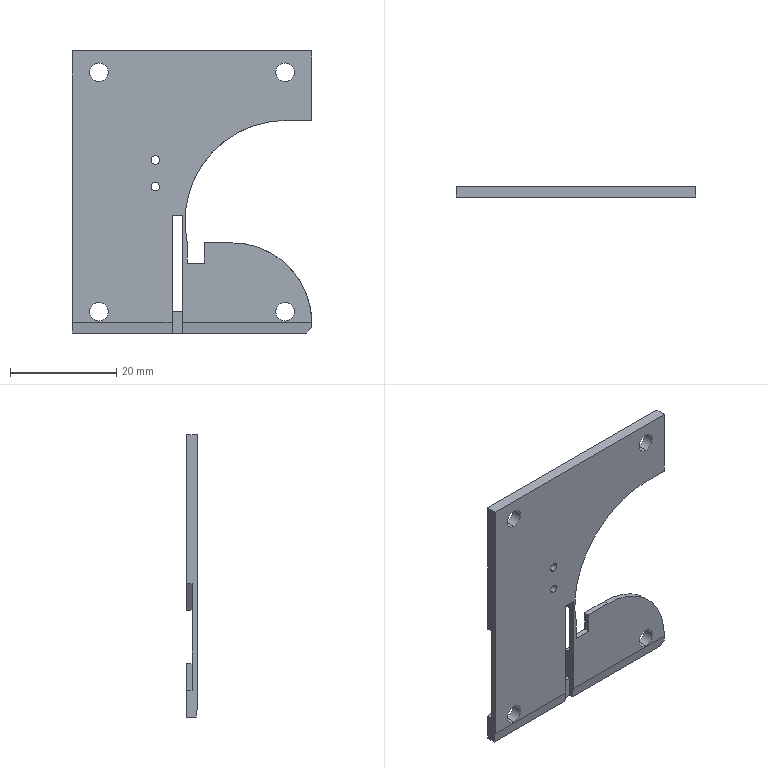Part | SolidWorks | features ICE 8, Chamfer 4, Extrusion 1, Fillet 1, HoleWzd 1 | 1 solid | 44 faces | box 45 x 2 x 53 mm | volume 3126 mm3 | plane 30 | cylinder 14 | commonest cylinder face diameters 3.5 x8 1.6 x4 30 x1 38 x1
STEP:
#1=CARTESIAN_POINT('',(-6.9,0.,6.7));
#2=VERTEX_POINT('',#1);
#3=CARTESIAN_POINT('',(-6.9,0.,8.3));
#4=VERTEX_POINT('',#3);
#5=CARTESIAN_POINT('',(-6.9,0.,7.5));
#6=DIRECTION('',(0.,1.,0.));
#7=DIRECTION('',(0.,0.,1.));
#8=AXIS2_PLACEMENT_3D('',#5,#6,#7);
#9=CIRCLE('',#8,0.8);
#10=EDGE_CURVE('',#2,#4,#9,.T.);
#11=ORIENTED_EDGE('',*,*,#10,.F.);
#12=CARTESIAN_POINT('',(-6.9,2.,6.7));
#13=VERTEX_POINT('',#12);
#14=CARTESIAN_POINT('',(-6.9,2.,6.7));
#15=DIRECTION('',(0.,1.,0.));
#16=VECTOR('',#15,1000.);
#17=LINE('',#14,#16);
#18=EDGE_CURVE('',#2,#13,#17,.T.);
#19=ORIENTED_EDGE('',*,*,#18,.T.);
#20=CARTESIAN_POINT('',(-6.9,2.,8.3));
#21=VERTEX_POINT('',#20);
#22=CARTESIAN_POINT('',(-6.9,2.,7.5));
#23=DIRECTION('',(0.,1.,0.));
#24=DIRECTION('',(0.,0.,1.));
#25=AXIS2_PLACEMENT_3D('',#22,#23,#24);
#26=CIRCLE('',#25,0.8);
#27=EDGE_CURVE('',#13,#21,#26,.T.);
#28=ORIENTED_EDGE('',*,*,#27,.T.);
#29=CARTESIAN_POINT('',(-6.9,2.,8.3));
#30=DIRECTION('',(0.,1.,0.));
#31=VECTOR('',#30,1000.);
#32=LINE('',#29,#31);
#33=EDGE_CURVE('',#4,#21,#32,.T.);
#34=ORIENTED_EDGE('',*,*,#33,.F.);
#35=EDGE_LOOP('',(#11,#19,#28,#34));
#36=FACE_OUTER_BOUND('',#35,.T.);
#37=CARTESIAN_POINT('',(-6.9,2.,7.5));
#38=DIRECTION('',(0.,1.,0.));
#39=DIRECTION('',(0.,0.,1.));
#40=AXIS2_PLACEMENT_3D('',#37,#38,#39);
#41=CYLINDRICAL_SURFACE('',#40,0.8);
#42=ADVANCED_FACE('',(#36),#41,.F.);
#43=CARTESIAN_POINT('',(-6.9,0.,1.7));
#44=VERTEX_POINT('',#43);
#45=CARTESIAN_POINT('',(-6.9,0.,3.3));
#46=VERTEX_POINT('',#45);
#47=CARTESIAN_POINT('',(-6.9,0.,2.5));
#48=DIRECTION('',(0.,1.,0.));
#49=DIRECTION('',(0.,0.,1.));
#50=AXIS2_PLACEMENT_3D('',#47,#48,#49);
#51=CIRCLE('',#50,0.8);
#52=EDGE_CURVE('',#44,#46,#51,.T.);
#53=ORIENTED_EDGE('',*,*,#52,.F.);
#54=CARTESIAN_POINT('',(-6.9,2.,1.7));
#55=VERTEX_POINT('',#54);
#56=CARTESIAN_POINT('',(-6.9,2.,1.7));
#57=DIRECTION('',(0.,1.,0.));
#58=VECTOR('',#57,1000.);
#59=LINE('',#56,#58);
#60=EDGE_CURVE('',#44,#55,#59,.T.);
#61=ORIENTED_EDGE('',*,*,#60,.T.);
#62=CARTESIAN_POINT('',(-6.9,2.,3.3));
#63=VERTEX_POINT('',#62);
#64=CARTESIAN_POINT('',(-6.9,2.,2.5));
#65=DIRECTION('',(0.,1.,0.));
#66=DIRECTION('',(0.,0.,1.));
#67=AXIS2_PLACEMENT_3D('',#64,#65,#66);
#68=CIRCLE('',#67,0.8);
#69=EDGE_CURVE('',#55,#63,#68,.T.);
#70=ORIENTED_EDGE('',*,*,#69,.T.);
#71=CARTESIAN_POINT('',(-6.9,2.,3.3));
#72=DIRECTION('',(0.,1.,0.));
#73=VECTOR('',#72,1000.);
#74=LINE('',#71,#73);
#75=EDGE_CURVE('',#46,#63,#74,.T.);
#76=ORIENTED_EDGE('',*,*,#75,.F.);
#77=EDGE_LOOP('',(#53,#61,#70,#76));
#78=FACE_OUTER_BOUND('',#77,.T.);
#79=CARTESIAN_POINT('',(-6.9,2.,2.5));
#80=DIRECTION('',(0.,1.,0.));
#81=DIRECTION('',(0.,0.,1.));
#82=AXIS2_PLACEMENT_3D('',#79,#80,#81);
#83=CYLINDRICAL_SURFACE('',#82,0.8);
#84=ADVANCED_FACE('',(#78),#83,.F.);
#85=CARTESIAN_POINT('',(-17.5,0.,22.25));
#86=VERTEX_POINT('',#85);
#87=CARTESIAN_POINT('',(-17.5,0.,25.75));
#88=VERTEX_POINT('',#87);
#89=CARTESIAN_POINT('',(-17.5,0.,24.));
#90=DIRECTION('',(0.,1.,0.));
#91=DIRECTION('',(0.,0.,-1.));
#92=AXIS2_PLACEMENT_3D('',#89,#90,#91);
#93=CIRCLE('',#92,1.75);
#94=EDGE_CURVE('',#86,#88,#93,.T.);
#95=ORIENTED_EDGE('',*,*,#94,.F.);
#96=CARTESIAN_POINT('',(-17.5,2.,22.25));
#97=VERTEX_POINT('',#96);
#98=CARTESIAN_POINT('',(-17.5,0.,22.25));
#99=DIRECTION('',(0.,1.,0.));
#100=VECTOR('',#99,1000.);
#101=LINE('',#98,#100);
#102=EDGE_CURVE('',#86,#97,#101,.T.);
#103=ORIENTED_EDGE('',*,*,#102,.T.);
#104=CARTESIAN_POINT('',(-17.5,2.,25.75));
#105=VERTEX_POINT('',#104);
#106=CARTESIAN_POINT('',(-17.5,2.,24.));
#107=DIRECTION('',(0.,1.,0.));
#108=DIRECTION('',(0.,0.,-1.));
#109=AXIS2_PLACEMENT_3D('',#106,#107,#108);
#110=CIRCLE('',#109,1.75);
#111=EDGE_CURVE('',#97,#105,#110,.T.);
#112=ORIENTED_EDGE('',*,*,#111,.T.);
#113=CARTESIAN_POINT('',(-17.5,0.,25.75));
#114=DIRECTION('',(0.,1.,0.));
#115=VECTOR('',#114,1000.);
#116=LINE('',#113,#115);
#117=EDGE_CURVE('',#88,#105,#116,.T.);
#118=ORIENTED_EDGE('',*,*,#117,.F.);
#119=EDGE_LOOP('',(#95,#103,#112,#118));
#120=FACE_OUTER_BOUND('',#119,.T.);
#121=CARTESIAN_POINT('',(-17.5,0.,24.));
#122=DIRECTION('',(0.,1.,0.));
#123=DIRECTION('',(0.,0.,1.));
#124=AXIS2_PLACEMENT_3D('',#121,#122,#123);
#125=CYLINDRICAL_SURFACE('',#124,1.75);
#126=ADVANCED_FACE('',(#120),#125,.F.);
#127=CARTESIAN_POINT('',(17.5,0.,22.25));
#128=VERTEX_POINT('',#127);
#129=CARTESIAN_POINT('',(17.5,0.,25.75));
#130=VERTEX_POINT('',#129);
#131=CARTESIAN_POINT('',(17.5,0.,24.));
#132=DIRECTION('',(0.,1.,0.));
#133=DIRECTION('',(0.,0.,1.));
#134=AXIS2_PLACEMENT_3D('',#131,#132,#133);
#135=CIRCLE('',#134,1.75);
#136=EDGE_CURVE('',#128,#130,#135,.T.);
#137=ORIENTED_EDGE('',*,*,#136,.F.);
#138=CARTESIAN_POINT('',(17.5,2.,22.25));
#139=VERTEX_POINT('',#138);
#140=CARTESIAN_POINT('',(17.5,0.,22.25));
#141=DIRECTION('',(0.,1.,0.));
#142=VECTOR('',#141,1000.);
#143=LINE('',#140,#142);
#144=EDGE_CURVE('',#128,#139,#143,.T.);
#145=ORIENTED_EDGE('',*,*,#144,.T.);
#146=CARTESIAN_POINT('',(17.5,2.,25.75));
#147=VERTEX_POINT('',#146);
#148=CARTESIAN_POINT('',(17.5,2.,24.));
#149=DIRECTION('',(0.,1.,0.));
#150=DIRECTION('',(0.,0.,1.));
#151=AXIS2_PLACEMENT_3D('',#148,#149,#150);
#152=CIRCLE('',#151,1.75);
#153=EDGE_CURVE('',#139,#147,#152,.T.);
#154=ORIENTED_EDGE('',*,*,#153,.T.);
#155=CARTESIAN_POINT('',(17.5,0.,25.75));
#156=DIRECTION('',(0.,1.,0.));
#157=VECTOR('',#156,1000.);
#158=LINE('',#155,#157);
#159=EDGE_CURVE('',#130,#147,#158,.T.);
#160=ORIENTED_EDGE('',*,*,#159,.F.);
#161=EDGE_LOOP('',(#137,#145,#154,#160));
#162=FACE_OUTER_BOUND('',#161,.T.);
#163=CARTESIAN_POINT('',(17.5,0.,24.));
#164=DIRECTION('',(0.,1.,0.));
#165=DIRECTION('',(0.,0.,1.));
#166=AXIS2_PLACEMENT_3D('',#163,#164,#165);
#167=CYLINDRICAL_SURFACE('',#166,1.75);
#168=ADVANCED_FACE('',(#162),#167,.F.);
#169=CARTESIAN_POINT('',(17.5,0.,-22.75));
#170=VERTEX_POINT('',#169);
#171=CARTESIAN_POINT('',(17.5,0.,-19.25));
#172=VERTEX_POINT('',#171);
#173=CARTESIAN_POINT('',(17.5,0.,-21.));
#174=DIRECTION('',(0.,1.,0.));
#175=DIRECTION('',(0.,0.,-1.));
#176=AXIS2_PLACEMENT_3D('',#173,#174,#175);
#177=CIRCLE('',#176,1.75);
#178=EDGE_CURVE('',#170,#172,#177,.T.);
#179=ORIENTED_EDGE('',*,*,#178,.F.);
#180=CARTESIAN_POINT('',(17.5,2.,-22.75));
#181=VERTEX_POINT('',#180);
#182=CARTESIAN_POINT('',(17.5,0.,-22.75));
#183=DIRECTION('',(0.,1.,0.));
#184=VECTOR('',#183,1000.);
#185=LINE('',#182,#184);
#186=EDGE_CURVE('',#170,#181,#185,.T.);
#187=ORIENTED_EDGE('',*,*,#186,.T.);
#188=CARTESIAN_POINT('',(17.5,2.,-19.25));
#189=VERTEX_POINT('',#188);
#190=CARTESIAN_POINT('',(17.5,2.,-21.));
#191=DIRECTION('',(0.,1.,0.));
#192=DIRECTION('',(0.,0.,-1.));
#193=AXIS2_PLACEMENT_3D('',#190,#191,#192);
#194=CIRCLE('',#193,1.75);
#195=EDGE_CURVE('',#181,#189,#194,.T.);
#196=ORIENTED_EDGE('',*,*,#195,.T.);
#197=CARTESIAN_POINT('',(17.5,0.,-19.25));
#198=DIRECTION('',(0.,1.,0.));
#199=VECTOR('',#198,1000.);
#200=LINE('',#197,#199);
#201=EDGE_CURVE('',#172,#189,#200,.T.);
#202=ORIENTED_EDGE('',*,*,#201,.F.);
#203=EDGE_LOOP('',(#179,#187,#196,#202));
#204=FACE_OUTER_BOUND('',#203,.T.);
#205=CARTESIAN_POINT('',(17.5,0.,-21.));
#206=DIRECTION('',(0.,1.,0.));
#207=DIRECTION('',(0.,0.,1.));
#208=AXIS2_PLACEMENT_3D('',#205,#206,#207);
#209=CYLINDRICAL_SURFACE('',#208,1.75);
#210=ADVANCED_FACE('',(#204),#209,.F.);
#211=CARTESIAN_POINT('',(-17.5,0.,-22.75));
#212=VERTEX_POINT('',#211);
#213=CARTESIAN_POINT('',(-17.5,0.,-19.25));
#214=VERTEX_POINT('',#213);
#215=CARTESIAN_POINT('',(-17.5,0.,-21.));
#216=DIRECTION('',(0.,1.,0.));
#217=DIRECTION('',(0.,0.,1.));
#218=AXIS2_PLACEMENT_3D('',#215,#216,#217);
#219=CIRCLE('',#218,1.75);
#220=EDGE_CURVE('',#212,#214,#219,.T.);
#221=ORIENTED_EDGE('',*,*,#220,.F.);
#222=CARTESIAN_POINT('',(-17.5,2.,-22.75));
#223=VERTEX_POINT('',#222);
#224=CARTESIAN_POINT('',(-17.5,0.,-22.75));
#225=DIRECTION('',(0.,1.,0.));
#226=VECTOR('',#225,1000.);
#227=LINE('',#224,#226);
#228=EDGE_CURVE('',#212,#223,#227,.T.);
#229=ORIENTED_EDGE('',*,*,#228,.T.);
#230=CARTESIAN_POINT('',(-17.5,2.,-19.25));
#231=VERTEX_POINT('',#230);
#232=CARTESIAN_POINT('',(-17.5,2.,-21.));
#233=DIRECTION('',(0.,1.,0.));
#234=DIRECTION('',(0.,0.,1.));
#235=AXIS2_PLACEMENT_3D('',#232,#233,#234);
#236=CIRCLE('',#235,1.75);
#237=EDGE_CURVE('',#223,#231,#236,.T.);
#238=ORIENTED_EDGE('',*,*,#237,.T.);
#239=CARTESIAN_POINT('',(-17.5,0.,-19.25));
#240=DIRECTION('',(0.,1.,0.));
#241=VECTOR('',#240,1000.);
#242=LINE('',#239,#241);
#243=EDGE_CURVE('',#214,#231,#242,.T.);
#244=ORIENTED_EDGE('',*,*,#243,.F.);
#245=EDGE_LOOP('',(#221,#229,#238,#244));
#246=FACE_OUTER_BOUND('',#245,.T.);
#247=CARTESIAN_POINT('',(-17.5,0.,-21.));
#248=DIRECTION('',(0.,1.,0.));
#249=DIRECTION('',(0.,0.,1.));
#250=AXIS2_PLACEMENT_3D('',#247,#248,#249);
#251=CYLINDRICAL_SURFACE('',#250,1.75);
#252=ADVANCED_FACE('',(#246),#251,.F.);
#253=CARTESIAN_POINT('',(-6.9,2.,7.5));
#254=DIRECTION('',(0.,1.,0.));
#255=DIRECTION('',(0.,0.,1.));
#256=AXIS2_PLACEMENT_3D('',#253,#254,#255);
#257=CIRCLE('',#256,0.8);
#258=EDGE_CURVE('',#21,#13,#257,.T.);
#259=ORIENTED_EDGE('',*,*,#258,.F.);
#260=ORIENTED_EDGE('',*,*,#27,.F.);
#261=EDGE_LOOP('',(#259,#260));
#262=FACE_BOUND('',#261,.T.);
#263=CARTESIAN_POINT('',(-6.9,2.,2.5));
#264=DIRECTION('',(0.,1.,0.));
#265=DIRECTION('',(0.,0.,1.));
#266=AXIS2_PLACEMENT_3D('',#263,#264,#265);
#267=CIRCLE('',#266,0.8);
#268=EDGE_CURVE('',#63,#55,#267,.T.);
#269=ORIENTED_EDGE('',*,*,#268,.F.);
#270=ORIENTED_EDGE('',*,*,#69,.F.);
#271=EDGE_LOOP('',(#269,#270));
#272=FACE_BOUND('',#271,.T.);
#273=CARTESIAN_POINT('',(17.674,2.,14.95));
#274=VERTEX_POINT('',#273);
#275=CARTESIAN_POINT('',(22.5,2.,14.95));
#276=VERTEX_POINT('',#275);
#277=CARTESIAN_POINT('',(17.674,2.,14.95));
#278=DIRECTION('',(1.,0.,0.));
#279=VECTOR('',#278,1000.);
#280=LINE('',#277,#279);
#281=EDGE_CURVE('',#274,#276,#280,.T.);
#282=ORIENTED_EDGE('',*,*,#281,.F.);
#283=CARTESIAN_POINT('',(-1.304,2.,-4.95));
#284=VERTEX_POINT('',#283);
#285=CARTESIAN_POINT('',(17.674,2.,-4.05));
#286=DIRECTION('',(0.,1.,0.));
#287=DIRECTION('',(0.,0.,1.));
#288=AXIS2_PLACEMENT_3D('',#285,#286,#287);
#289=CIRCLE('',#288,19.);
#290=EDGE_CURVE('',#284,#274,#289,.T.);
#291=ORIENTED_EDGE('',*,*,#290,.F.);
#292=CARTESIAN_POINT('',(-1.75,2.,-4.95));
#293=VERTEX_POINT('',#292);
#294=CARTESIAN_POINT('',(-24.3,2.,-4.95));
#295=DIRECTION('',(1.,0.,0.));
#296=VECTOR('',#295,1000.);
#297=LINE('',#294,#296);
#298=EDGE_CURVE('',#293,#284,#297,.T.);
#299=ORIENTED_EDGE('',*,*,#298,.F.);
#300=CARTESIAN_POINT('',(-1.75,2.,-3.));
#301=VERTEX_POINT('',#300);
#302=CARTESIAN_POINT('',(-1.75,2.,-21.));
#303=DIRECTION('',(0.,0.,-1.));
#304=VECTOR('',#303,1000.);
#305=LINE('',#302,#304);
#306=EDGE_CURVE('',#301,#293,#305,.T.);
#307=ORIENTED_EDGE('',*,*,#306,.F.);
#308=CARTESIAN_POINT('',(-3.75,2.,-3.));
#309=VERTEX_POINT('',#308);
#310=CARTESIAN_POINT('',(-3.75,2.,-3.));
#311=DIRECTION('',(1.,0.,0.));
#312=VECTOR('',#311,1000.);
#313=LINE('',#310,#312);
#314=EDGE_CURVE('',#309,#301,#313,.T.);
#315=ORIENTED_EDGE('',*,*,#314,.F.);
#316=CARTESIAN_POINT('',(-3.75,2.,-4.95));
#317=VERTEX_POINT('',#316);
#318=CARTESIAN_POINT('',(-3.75,2.,-21.));
#319=DIRECTION('',(0.,0.,1.));
#320=VECTOR('',#319,1000.);
#321=LINE('',#318,#320);
#322=EDGE_CURVE('',#317,#309,#321,.T.);
#323=ORIENTED_EDGE('',*,*,#322,.F.);
#324=CARTESIAN_POINT('',(-7.5,2.,-4.95));
#325=VERTEX_POINT('',#324);
#326=CARTESIAN_POINT('',(-24.3,2.,-4.95));
#327=DIRECTION('',(1.,0.,0.));
#328=VECTOR('',#327,1000.);
#329=LINE('',#326,#328);
#330=EDGE_CURVE('',#325,#317,#329,.T.);
#331=ORIENTED_EDGE('',*,*,#330,.F.);
#332=CARTESIAN_POINT('',(-22.5,2.,0.05));
#333=VERTEX_POINT('',#332);
#334=CARTESIAN_POINT('',(-2.235,2.,-6.705));
#335=DIRECTION('',(-0.9487,0.,0.3162));
#336=VECTOR('',#335,1000.);
#337=LINE('',#334,#336);
#338=EDGE_CURVE('',#325,#333,#337,.T.);
#339=ORIENTED_EDGE('',*,*,#338,.T.);
#340=CARTESIAN_POINT('',(-22.5,2.,28.));
#341=VERTEX_POINT('',#340);
#342=CARTESIAN_POINT('',(-22.5,2.,-25.));
#343=DIRECTION('',(0.,0.,1.));
#344=VECTOR('',#343,1000.);
#345=LINE('',#342,#344);
#346=EDGE_CURVE('',#333,#341,#345,.T.);
#347=ORIENTED_EDGE('',*,*,#346,.T.);
#348=CARTESIAN_POINT('',(22.5,2.,28.));
#349=VERTEX_POINT('',#348);
#350=CARTESIAN_POINT('',(-22.5,2.,28.));
#351=DIRECTION('',(-1.,0.,0.));
#352=VECTOR('',#351,1000.);
#353=LINE('',#350,#352);
#354=EDGE_CURVE('',#349,#341,#353,.T.);
#355=ORIENTED_EDGE('',*,*,#354,.F.);
#356=CARTESIAN_POINT('',(22.5,2.,-25.));
#357=DIRECTION('',(0.,0.,-1.));
#358=VECTOR('',#357,1000.);
#359=LINE('',#356,#358);
#360=EDGE_CURVE('',#349,#276,#359,.T.);
#361=ORIENTED_EDGE('',*,*,#360,.T.);
#362=EDGE_LOOP('',(#282,#291,#299,#307,#315,#323,#331,#339,#347,#355,#361));
#363=FACE_OUTER_BOUND('',#362,.T.);
#364=CARTESIAN_POINT('',(-17.5,2.,24.));
#365=DIRECTION('',(0.,1.,0.));
#366=DIRECTION('',(0.,0.,-1.));
#367=AXIS2_PLACEMENT_3D('',#364,#365,#366);
#368=CIRCLE('',#367,1.75);
#369=EDGE_CURVE('',#105,#97,#368,.T.);
#370=ORIENTED_EDGE('',*,*,#369,.F.);
#371=ORIENTED_EDGE('',*,*,#111,.F.);
#372=EDGE_LOOP('',(#370,#371));
#373=FACE_BOUND('',#372,.T.);
#374=CARTESIAN_POINT('',(17.5,2.,24.));
#375=DIRECTION('',(0.,1.,0.));
#376=DIRECTION('',(0.,0.,1.));
#377=AXIS2_PLACEMENT_3D('',#374,#375,#376);
#378=CIRCLE('',#377,1.75);
#379=EDGE_CURVE('',#147,#139,#378,.T.);
#380=ORIENTED_EDGE('',*,*,#379,.F.);
#381=ORIENTED_EDGE('',*,*,#153,.F.);
#382=EDGE_LOOP('',(#380,#381));
#383=FACE_BOUND('',#382,.T.);
#384=CARTESIAN_POINT('',(0.,2.,0.));
#385=DIRECTION('',(0.,1.,0.));
#386=DIRECTION('',(0.,0.,1.));
#387=AXIS2_PLACEMENT_3D('',#384,#385,#386);
#388=PLANE('',#387);
#389=ADVANCED_FACE('',(#262,#272,#363,#373,#383),#388,.T.);
#390=CARTESIAN_POINT('',(22.5,0.,28.));
#391=VERTEX_POINT('',#390);
#392=CARTESIAN_POINT('',(22.5,0.,14.95));
#393=VERTEX_POINT('',#392);
#394=CARTESIAN_POINT('',(22.5,0.,-25.));
#395=DIRECTION('',(0.,0.,-1.));
#396=VECTOR('',#395,1000.);
#397=LINE('',#394,#396);
#398=EDGE_CURVE('',#391,#393,#397,.T.);
#399=ORIENTED_EDGE('',*,*,#398,.T.);
#400=CARTESIAN_POINT('',(22.5,0.,14.95));
#401=DIRECTION('',(0.,1.,0.));
#402=VECTOR('',#401,1000.);
#403=LINE('',#400,#402);
#404=EDGE_CURVE('',#393,#276,#403,.T.);
#405=ORIENTED_EDGE('',*,*,#404,.T.);
#406=ORIENTED_EDGE('',*,*,#360,.F.);
#407=CARTESIAN_POINT('',(22.5,2.,28.));
#408=DIRECTION('',(0.,1.,0.));
#409=VECTOR('',#408,1000.);
#410=LINE('',#407,#409);
#411=EDGE_CURVE('',#391,#349,#410,.T.);
#412=ORIENTED_EDGE('',*,*,#411,.F.);
#413=EDGE_LOOP('',(#399,#405,#406,#412));
#414=FACE_OUTER_BOUND('',#413,.T.);
#415=CARTESIAN_POINT('',(22.5,2.,-25.));
#416=DIRECTION('',(-1.,0.,0.));
#417=DIRECTION('',(0.,0.,1.));
#418=AXIS2_PLACEMENT_3D('',#415,#416,#417);
#419=PLANE('',#418);
#420=ADVANCED_FACE('',(#414),#419,.F.);
#421=CARTESIAN_POINT('',(-1.75,1.,-21.));
#422=VERTEX_POINT('',#421);
#423=CARTESIAN_POINT('',(-3.75,1.,-21.));
#424=VERTEX_POINT('',#423);
#425=CARTESIAN_POINT('',(-3.75,1.,-21.));
#426=DIRECTION('',(-1.,0.,0.));
#427=VECTOR('',#426,1000.);
#428=LINE('',#425,#427);
#429=EDGE_CURVE('',#422,#424,#428,.T.);
#430=ORIENTED_EDGE('',*,*,#429,.F.);
#431=CARTESIAN_POINT('',(-1.75,2.,-21.));
#432=VERTEX_POINT('',#431);
#433=CARTESIAN_POINT('',(-1.75,0.,-21.));
#434=DIRECTION('',(0.,1.,0.));
#435=VECTOR('',#434,1000.);
#436=LINE('',#433,#435);
#437=EDGE_CURVE('',#422,#432,#436,.T.);
#438=ORIENTED_EDGE('',*,*,#437,.T.);
#439=CARTESIAN_POINT('',(-3.75,2.,-21.));
#440=VERTEX_POINT('',#439);
#441=CARTESIAN_POINT('',(-3.75,2.,-21.));
#442=DIRECTION('',(-1.,0.,0.));
#443=VECTOR('',#442,1000.);
#444=LINE('',#441,#443);
#445=EDGE_CURVE('',#432,#440,#444,.T.);
#446=ORIENTED_EDGE('',*,*,#445,.T.);
#447=CARTESIAN_POINT('',(-3.75,0.,-21.));
#448=DIRECTION('',(0.,1.,0.));
#449=VECTOR('',#448,1000.);
#450=LINE('',#447,#449);
#451=EDGE_CURVE('',#424,#440,#450,.T.);
#452=ORIENTED_EDGE('',*,*,#451,.F.);
#453=EDGE_LOOP('',(#430,#438,#446,#452));
#454=FACE_OUTER_BOUND('',#453,.T.);
#455=CARTESIAN_POINT('',(-3.75,0.,-21.));
#456=DIRECTION('',(0.,0.,-1.));
#457=DIRECTION('',(-1.,0.,0.));
#458=AXIS2_PLACEMENT_3D('',#455,#456,#457);
#459=PLANE('',#458);
#460=ADVANCED_FACE('',(#454),#459,.F.);
#461=CARTESIAN_POINT('',(22.5,0.005,-23.05));
#462=VERTEX_POINT('',#461);
#463=CARTESIAN_POINT('',(22.5,0.1,-24.));
#464=VERTEX_POINT('',#463);
#465=CARTESIAN_POINT('',(22.5,0.2,-25.));
#466=DIRECTION('',(0.,0.0995,-0.995));
#467=VECTOR('',#466,1000.);
#468=LINE('',#465,#467);
#469=EDGE_CURVE('',#462,#464,#468,.T.);
#470=ORIENTED_EDGE('',*,*,#469,.T.);
#471=CARTESIAN_POINT('',(22.5,2.,-24.));
#472=VERTEX_POINT('',#471);
#473=CARTESIAN_POINT('',(22.5,2.,-24.));
#474=DIRECTION('',(0.,1.,0.));
#475=VECTOR('',#474,1000.);
#476=LINE('',#473,#475);
#477=EDGE_CURVE('',#464,#472,#476,.T.);
#478=ORIENTED_EDGE('',*,*,#477,.T.);
#479=CARTESIAN_POINT('',(22.5,2.,-23.05));
#480=VERTEX_POINT('',#479);
#481=CARTESIAN_POINT('',(22.5,2.,-25.));
#482=DIRECTION('',(0.,0.,-1.));
#483=VECTOR('',#482,1000.);
#484=LINE('',#481,#483);
#485=EDGE_CURVE('',#480,#472,#484,.T.);
#486=ORIENTED_EDGE('',*,*,#485,.F.);
#487=CARTESIAN_POINT('',(22.5,2.,-23.05));
#488=DIRECTION('',(0.,-1.,0.));
#489=VECTOR('',#488,1000.);
#490=LINE('',#487,#489);
#491=EDGE_CURVE('',#480,#462,#490,.T.);
#492=ORIENTED_EDGE('',*,*,#491,.T.);
#493=EDGE_LOOP('',(#470,#478,#486,#492));
#494=FACE_OUTER_BOUND('',#493,.T.);
#495=CARTESIAN_POINT('',(22.5,2.,-25.));
#496=DIRECTION('',(-1.,0.,0.));
#497=DIRECTION('',(0.,0.,1.));
#498=AXIS2_PLACEMENT_3D('',#495,#496,#497);
#499=PLANE('',#498);
#500=ADVANCED_FACE('',(#494),#499,.F.);
#501=CARTESIAN_POINT('',(21.5,2.,-25.));
#502=VERTEX_POINT('',#501);
#503=CARTESIAN_POINT('',(-22.5,2.,-25.));
#504=VERTEX_POINT('',#503);
#505=CARTESIAN_POINT('',(-22.5,2.,-25.));
#506=DIRECTION('',(-1.,0.,0.));
#507=VECTOR('',#506,1000.);
#508=LINE('',#505,#507);
#509=EDGE_CURVE('',#502,#504,#508,.T.);
#510=ORIENTED_EDGE('',*,*,#509,.F.);
#511=CARTESIAN_POINT('',(21.5,0.2,-25.));
#512=VERTEX_POINT('',#511);
#513=CARTESIAN_POINT('',(21.5,2.,-25.));
#514=DIRECTION('',(0.,-1.,0.));
#515=VECTOR('',#514,1000.);
#516=LINE('',#513,#515);
#517=EDGE_CURVE('',#502,#512,#516,.T.);
#518=ORIENTED_EDGE('',*,*,#517,.T.);
#519=CARTESIAN_POINT('',(-1.75,0.2,-25.));
#520=VERTEX_POINT('',#519);
#521=CARTESIAN_POINT('',(-22.5,0.2,-25.));
#522=DIRECTION('',(-1.,0.,0.));
#523=VECTOR('',#522,1000.);
#524=LINE('',#521,#523);
#525=EDGE_CURVE('',#512,#520,#524,.T.);
#526=ORIENTED_EDGE('',*,*,#525,.T.);
#527=CARTESIAN_POINT('',(-1.75,1.,-25.));
#528=VERTEX_POINT('',#527);
#529=CARTESIAN_POINT('',(-1.75,1.,-25.));
#530=DIRECTION('',(0.,-1.,0.));
#531=VECTOR('',#530,1000.);
#532=LINE('',#529,#531);
#533=EDGE_CURVE('',#528,#520,#532,.T.);
#534=ORIENTED_EDGE('',*,*,#533,.F.);
#535=CARTESIAN_POINT('',(-3.75,1.,-25.));
#536=VERTEX_POINT('',#535);
#537=CARTESIAN_POINT('',(-3.75,1.,-25.));
#538=DIRECTION('',(1.,0.,0.));
#539=VECTOR('',#538,1000.);
#540=LINE('',#537,#539);
#541=EDGE_CURVE('',#536,#528,#540,.T.);
#542=ORIENTED_EDGE('',*,*,#541,.F.);
#543=CARTESIAN_POINT('',(-3.75,0.2,-25.));
#544=VERTEX_POINT('',#543);
#545=CARTESIAN_POINT('',(-3.75,1.,-25.));
#546=DIRECTION('',(0.,-1.,0.));
#547=VECTOR('',#546,1000.);
#548=LINE('',#545,#547);
#549=EDGE_CURVE('',#536,#544,#548,.T.);
#550=ORIENTED_EDGE('',*,*,#549,.T.);
#551=CARTESIAN_POINT('',(-22.5,0.2,-25.));
#552=VERTEX_POINT('',#551);
#553=CARTESIAN_POINT('',(-22.5,0.2,-25.));
#554=DIRECTION('',(-1.,0.,0.));
#555=VECTOR('',#554,1000.);
#556=LINE('',#553,#555);
#557=EDGE_CURVE('',#544,#552,#556,.T.);
#558=ORIENTED_EDGE('',*,*,#557,.T.);
#559=CARTESIAN_POINT('',(-22.5,2.,-25.));
#560=DIRECTION('',(0.,-1.,0.));
#561=VECTOR('',#560,1000.);
#562=LINE('',#559,#561);
#563=EDGE_CURVE('',#504,#552,#562,.T.);
#564=ORIENTED_EDGE('',*,*,#563,.F.);
#565=EDGE_LOOP('',(#510,#518,#526,#534,#542,#550,#558,#564));
#566=FACE_OUTER_BOUND('',#565,.T.);
#567=CARTESIAN_POINT('',(-22.5,2.,-25.));
#568=DIRECTION('',(0.,0.,1.));
#569=DIRECTION('',(1.,0.,0.));
#570=AXIS2_PLACEMENT_3D('',#567,#568,#569);
#571=PLANE('',#570);
#572=ADVANCED_FACE('',(#566),#571,.F.);
#573=ORIENTED_EDGE('',*,*,#563,.T.);
#574=CARTESIAN_POINT('',(-22.5,0.,-23.));
#575=VERTEX_POINT('',#574);
#576=CARTESIAN_POINT('',(-22.5,0.2,-25.));
#577=DIRECTION('',(0.,-0.0995,0.995));
#578=VECTOR('',#577,1000.);
#579=LINE('',#576,#578);
#580=EDGE_CURVE('',#552,#575,#579,.T.);
#581=ORIENTED_EDGE('',*,*,#580,.T.);
#582=CARTESIAN_POINT('',(-22.5,0.,28.));
#583=VERTEX_POINT('',#582);
#584=CARTESIAN_POINT('',(-22.5,0.,-25.));
#585=DIRECTION('',(0.,0.,1.));
#586=VECTOR('',#585,1000.);
#587=LINE('',#584,#586);
#588=EDGE_CURVE('',#575,#583,#587,.T.);
#589=ORIENTED_EDGE('',*,*,#588,.T.);
#590=CARTESIAN_POINT('',(-22.5,2.,28.));
#591=DIRECTION('',(0.,-1.,0.));
#592=VECTOR('',#591,1000.);
#593=LINE('',#590,#592);
#594=EDGE_CURVE('',#341,#583,#593,.T.);
#595=ORIENTED_EDGE('',*,*,#594,.F.);
#596=ORIENTED_EDGE('',*,*,#346,.F.);
#597=CARTESIAN_POINT('',(-22.5,1.,0.05));
#598=VERTEX_POINT('',#597);
#599=CARTESIAN_POINT('',(-22.5,2.,0.05));
#600=DIRECTION('',(0.,-1.,0.));
#601=VECTOR('',#600,1000.);
#602=LINE('',#599,#601);
#603=EDGE_CURVE('',#333,#598,#602,.T.);
#604=ORIENTED_EDGE('',*,*,#603,.T.);
#605=CARTESIAN_POINT('',(-22.5,1.,-19.95));
#606=VERTEX_POINT('',#605);
#607=CARTESIAN_POINT('',(-22.5,1.,-25.));
#608=DIRECTION('',(0.,0.,-1.));
#609=VECTOR('',#608,1000.);
#610=LINE('',#607,#609);
#611=EDGE_CURVE('',#598,#606,#610,.T.);
#612=ORIENTED_EDGE('',*,*,#611,.T.);
#613=CARTESIAN_POINT('',(-22.5,2.,-19.95));
#614=VERTEX_POINT('',#613);
#615=CARTESIAN_POINT('',(-22.5,2.,-19.95));
#616=DIRECTION('',(0.,1.,0.));
#617=VECTOR('',#616,1000.);
#618=LINE('',#615,#617);
#619=EDGE_CURVE('',#606,#614,#618,.T.);
#620=ORIENTED_EDGE('',*,*,#619,.T.);
#621=CARTESIAN_POINT('',(-22.5,2.,-25.));
#622=DIRECTION('',(0.,0.,1.));
#623=VECTOR('',#622,1000.);
#624=LINE('',#621,#623);
#625=EDGE_CURVE('',#504,#614,#624,.T.);
#626=ORIENTED_EDGE('',*,*,#625,.F.);
#627=EDGE_LOOP('',(#573,#581,#589,#595,#596,#604,#612,#620,#626));
#628=FACE_OUTER_BOUND('',#627,.T.);
#629=CARTESIAN_POINT('',(-22.5,2.,-25.));
#630=DIRECTION('',(1.,0.,0.));
#631=DIRECTION('',(0.,0.,-1.));
#632=AXIS2_PLACEMENT_3D('',#629,#630,#631);
#633=PLANE('',#632);
#634=ADVANCED_FACE('',(#628),#633,.F.);
#635=CARTESIAN_POINT('',(17.5,2.,-21.));
#636=DIRECTION('',(0.,1.,0.));
#637=DIRECTION('',(0.,0.,-1.));
#638=AXIS2_PLACEMENT_3D('',#635,#636,#637);
#639=CIRCLE('',#638,1.75);
#640=EDGE_CURVE('',#189,#181,#639,.T.);
#641=ORIENTED_EDGE('',*,*,#640,.F.);
#642=ORIENTED_EDGE('',*,*,#195,.F.);
#643=EDGE_LOOP('',(#641,#642));
#644=FACE_BOUND('',#643,.T.);
#645=CARTESIAN_POINT('',(-17.5,2.,-21.));
#646=DIRECTION('',(0.,1.,0.));
#647=DIRECTION('',(0.,0.,1.));
#648=AXIS2_PLACEMENT_3D('',#645,#646,#647);
#649=CIRCLE('',#648,1.75);
#650=EDGE_CURVE('',#231,#223,#649,.T.);
#651=ORIENTED_EDGE('',*,*,#650,.F.);
#652=ORIENTED_EDGE('',*,*,#237,.F.);
#653=EDGE_LOOP('',(#651,#652));
#654=FACE_BOUND('',#653,.T.);
#655=ORIENTED_EDGE('',*,*,#485,.T.);
#656=CARTESIAN_POINT('',(23.25,2.,-23.25));
#657=DIRECTION('',(-0.7071,0.,-0.7071));
#658=VECTOR('',#657,1000.);
#659=LINE('',#656,#658);
#660=EDGE_CURVE('',#472,#502,#659,.T.);
#661=ORIENTED_EDGE('',*,*,#660,.T.);
#662=ORIENTED_EDGE('',*,*,#509,.T.);
#663=ORIENTED_EDGE('',*,*,#625,.T.);
#664=CARTESIAN_POINT('',(-7.5,2.,-14.95));
#665=VERTEX_POINT('',#664);
#666=CARTESIAN_POINT('',(3.735,2.,-11.205));
#667=DIRECTION('',(0.9487,0.,0.3162));
#668=VECTOR('',#667,1000.);
#669=LINE('',#666,#668);
#670=EDGE_CURVE('',#614,#665,#669,.T.);
#671=ORIENTED_EDGE('',*,*,#670,.T.);
#672=CARTESIAN_POINT('',(-3.75,2.,-14.95));
#673=VERTEX_POINT('',#672);
#674=CARTESIAN_POINT('',(-24.3,2.,-14.95));
#675=DIRECTION('',(-1.,0.,0.));
#676=VECTOR('',#675,1000.);
#677=LINE('',#674,#676);
#678=EDGE_CURVE('',#673,#665,#677,.T.);
#679=ORIENTED_EDGE('',*,*,#678,.F.);
#680=CARTESIAN_POINT('',(-3.75,2.,-21.));
#681=DIRECTION('',(0.,0.,1.));
#682=VECTOR('',#681,1000.);
#683=LINE('',#680,#682);
#684=EDGE_CURVE('',#440,#673,#683,.T.);
#685=ORIENTED_EDGE('',*,*,#684,.F.);
#686=ORIENTED_EDGE('',*,*,#445,.F.);
#687=CARTESIAN_POINT('',(-1.75,2.,-14.95));
#688=VERTEX_POINT('',#687);
#689=CARTESIAN_POINT('',(-1.75,2.,-21.));
#690=DIRECTION('',(0.,0.,-1.));
#691=VECTOR('',#690,1000.);
#692=LINE('',#689,#691);
#693=EDGE_CURVE('',#688,#432,#692,.T.);
#694=ORIENTED_EDGE('',*,*,#693,.F.);
#695=CARTESIAN_POINT('',(7.5,2.,-14.95));
#696=VERTEX_POINT('',#695);
#697=CARTESIAN_POINT('',(-24.3,2.,-14.95));
#698=DIRECTION('',(-1.,0.,0.));
#699=VECTOR('',#698,1000.);
#700=LINE('',#697,#699);
#701=EDGE_CURVE('',#696,#688,#700,.T.);
#702=ORIENTED_EDGE('',*,*,#701,.F.);
#703=CARTESIAN_POINT('',(22.151,2.,-19.834));
#704=VERTEX_POINT('',#703);
#705=CARTESIAN_POINT('',(-3.735,2.,-11.205));
#706=DIRECTION('',(0.9487,0.,-0.3162));
#707=VECTOR('',#706,1000.);
#708=LINE('',#705,#707);
#709=EDGE_CURVE('',#696,#704,#708,.T.);
#710=ORIENTED_EDGE('',*,*,#709,.T.);
#711=CARTESIAN_POINT('',(7.5,2.,-23.05));
#712=DIRECTION('',(0.,1.,0.));
#713=DIRECTION('',(0.,0.,1.));
#714=AXIS2_PLACEMENT_3D('',#711,#712,#713);
#715=CIRCLE('',#714,15.);
#716=EDGE_CURVE('',#704,#480,#715,.T.);
#717=ORIENTED_EDGE('',*,*,#716,.T.);
#718=EDGE_LOOP('',(#655,#661,#662,#663,#671,#679,#685,#686,#694,#702,#710,#717));
#719=FACE_OUTER_BOUND('',#718,.T.);
#720=CARTESIAN_POINT('',(0.,2.,0.));
#721=DIRECTION('',(0.,1.,0.));
#722=DIRECTION('',(0.,0.,1.));
#723=AXIS2_PLACEMENT_3D('',#720,#721,#722);
#724=PLANE('',#723);
#725=ADVANCED_FACE('',(#644,#654,#719),#724,.T.);
#726=CARTESIAN_POINT('',(-6.9,0.,7.5));
#727=DIRECTION('',(0.,1.,0.));
#728=DIRECTION('',(0.,0.,1.));
#729=AXIS2_PLACEMENT_3D('',#726,#727,#728);
#730=CIRCLE('',#729,0.8);
#731=EDGE_CURVE('',#4,#2,#730,.T.);
#732=ORIENTED_EDGE('',*,*,#731,.T.);
#733=ORIENTED_EDGE('',*,*,#10,.T.);
#734=EDGE_LOOP('',(#732,#733));
#735=FACE_BOUND('',#734,.T.);
#736=CARTESIAN_POINT('',(-6.9,0.,2.5));
#737=DIRECTION('',(0.,1.,0.));
#738=DIRECTION('',(0.,0.,1.));
#739=AXIS2_PLACEMENT_3D('',#736,#737,#738);
#740=CIRCLE('',#739,0.8);
#741=EDGE_CURVE('',#46,#44,#740,.T.);
#742=ORIENTED_EDGE('',*,*,#741,.T.);
#743=ORIENTED_EDGE('',*,*,#52,.T.);
#744=EDGE_LOOP('',(#742,#743));
#745=FACE_BOUND('',#744,.T.);
#746=CARTESIAN_POINT('',(-17.5,0.,24.));
#747=DIRECTION('',(0.,1.,0.));
#748=DIRECTION('',(0.,0.,-1.));
#749=AXIS2_PLACEMENT_3D('',#746,#747,#748);
#750=CIRCLE('',#749,1.75);
#751=EDGE_CURVE('',#88,#86,#750,.T.);
#752=ORIENTED_EDGE('',*,*,#751,.T.);
#753=ORIENTED_EDGE('',*,*,#94,.T.);
#754=EDGE_LOOP('',(#752,#753));
#755=FACE_BOUND('',#754,.T.);
#756=CARTESIAN_POINT('',(17.5,0.,24.));
#757=DIRECTION('',(0.,1.,0.));
#758=DIRECTION('',(0.,0.,1.));
#759=AXIS2_PLACEMENT_3D('',#756,#757,#758);
#760=CIRCLE('',#759,1.75);
#761=EDGE_CURVE('',#130,#128,#760,.T.);
#762=ORIENTED_EDGE('',*,*,#761,.T.);
#763=ORIENTED_EDGE('',*,*,#136,.T.);
#764=EDGE_LOOP('',(#762,#763));
#765=FACE_BOUND('',#764,.T.);
#766=CARTESIAN_POINT('',(17.5,0.,-21.));
#767=DIRECTION('',(0.,1.,0.));
#768=DIRECTION('',(0.,0.,-1.));
#769=AXIS2_PLACEMENT_3D('',#766,#767,#768);
#770=CIRCLE('',#769,1.75);
#771=EDGE_CURVE('',#172,#170,#770,.T.);
#772=ORIENTED_EDGE('',*,*,#771,.T.);
#773=ORIENTED_EDGE('',*,*,#178,.T.);
#774=EDGE_LOOP('',(#772,#773));
#775=FACE_BOUND('',#774,.T.);
#776=CARTESIAN_POINT('',(-17.5,0.,-21.));
#777=DIRECTION('',(0.,1.,0.));
#778=DIRECTION('',(0.,0.,1.));
#779=AXIS2_PLACEMENT_3D('',#776,#777,#778);
#780=CIRCLE('',#779,1.75);
#781=EDGE_CURVE('',#214,#212,#780,.T.);
#782=ORIENTED_EDGE('',*,*,#781,.T.);
#783=ORIENTED_EDGE('',*,*,#220,.T.);
#784=EDGE_LOOP('',(#782,#783));
#785=FACE_BOUND('',#784,.T.);
#786=CARTESIAN_POINT('',(-0.9,0.,-8.05));
#787=VERTEX_POINT('',#786);
#788=CARTESIAN_POINT('',(17.674,0.,14.95));
#789=VERTEX_POINT('',#788);
#790=CARTESIAN_POINT('',(17.674,0.,-4.05));
#791=DIRECTION('',(0.,1.,0.));
#792=DIRECTION('',(0.,0.,1.));
#793=AXIS2_PLACEMENT_3D('',#790,#791,#792);
#794=CIRCLE('',#793,19.);
#795=EDGE_CURVE('',#787,#789,#794,.T.);
#796=ORIENTED_EDGE('',*,*,#795,.T.);
#797=CARTESIAN_POINT('',(17.674,0.,14.95));
#798=DIRECTION('',(1.,0.,0.));
#799=VECTOR('',#798,1000.);
#800=LINE('',#797,#799);
#801=EDGE_CURVE('',#789,#393,#800,.T.);
#802=ORIENTED_EDGE('',*,*,#801,.T.);
#803=ORIENTED_EDGE('',*,*,#398,.F.);
#804=CARTESIAN_POINT('',(-22.5,0.,28.));
#805=DIRECTION('',(1.,0.,0.));
#806=VECTOR('',#805,1000.);
#807=LINE('',#804,#806);
#808=EDGE_CURVE('',#583,#391,#807,.T.);
#809=ORIENTED_EDGE('',*,*,#808,.F.);
#810=ORIENTED_EDGE('',*,*,#588,.F.);
#811=CARTESIAN_POINT('',(-3.75,0.,-23.));
#812=VERTEX_POINT('',#811);
#813=CARTESIAN_POINT('',(0.,0.,-23.));
#814=DIRECTION('',(1.,0.,0.));
#815=VECTOR('',#814,1000.);
#816=LINE('',#813,#815);
#817=EDGE_CURVE('',#575,#812,#816,.T.);
#818=ORIENTED_EDGE('',*,*,#817,.T.);
#819=CARTESIAN_POINT('',(-3.75,0.,-3.));
#820=VERTEX_POINT('',#819);
#821=CARTESIAN_POINT('',(-3.75,0.,-21.));
#822=DIRECTION('',(0.,0.,1.));
#823=VECTOR('',#822,1000.);
#824=LINE('',#821,#823);
#825=EDGE_CURVE('',#812,#820,#824,.T.);
#826=ORIENTED_EDGE('',*,*,#825,.T.);
#827=CARTESIAN_POINT('',(-1.75,0.,-3.));
#828=VERTEX_POINT('',#827);
#829=CARTESIAN_POINT('',(-3.75,0.,-3.));
#830=DIRECTION('',(1.,0.,0.));
#831=VECTOR('',#830,1000.);
#832=LINE('',#829,#831);
#833=EDGE_CURVE('',#820,#828,#832,.T.);
#834=ORIENTED_EDGE('',*,*,#833,.T.);
#835=CARTESIAN_POINT('',(-1.75,0.,-23.));
#836=VERTEX_POINT('',#835);
#837=CARTESIAN_POINT('',(-1.75,0.,-21.));
#838=DIRECTION('',(0.,0.,-1.));
#839=VECTOR('',#838,1000.);
#840=LINE('',#837,#839);
#841=EDGE_CURVE('',#828,#836,#840,.T.);
#842=ORIENTED_EDGE('',*,*,#841,.T.);
#843=CARTESIAN_POINT('',(22.5,0.,-23.));
#844=VERTEX_POINT('',#843);
#845=CARTESIAN_POINT('',(0.,0.,-23.));
#846=DIRECTION('',(1.,0.,0.));
#847=VECTOR('',#846,1000.);
#848=LINE('',#845,#847);
#849=EDGE_CURVE('',#836,#844,#848,.T.);
#850=ORIENTED_EDGE('',*,*,#849,.T.);
#851=CARTESIAN_POINT('',(7.5,0.,-8.05));
#852=VERTEX_POINT('',#851);
#853=CARTESIAN_POINT('',(7.5,0.,-23.05));
#854=DIRECTION('',(0.,-1.,0.));
#855=DIRECTION('',(0.,0.,1.));
#856=AXIS2_PLACEMENT_3D('',#853,#854,#855);
#857=CIRCLE('',#856,15.);
#858=EDGE_CURVE('',#844,#852,#857,.T.);
#859=ORIENTED_EDGE('',*,*,#858,.T.);
#860=CARTESIAN_POINT('',(2.3,0.,-8.05));
#861=VERTEX_POINT('',#860);
#862=CARTESIAN_POINT('',(0.,0.,-8.05));
#863=DIRECTION('',(-1.,0.,0.));
#864=VECTOR('',#863,1000.);
#865=LINE('',#862,#864);
#866=EDGE_CURVE('',#852,#861,#865,.T.);
#867=ORIENTED_EDGE('',*,*,#866,.T.);
#868=CARTESIAN_POINT('',(2.3,0.,-11.85));
#869=VERTEX_POINT('',#868);
#870=CARTESIAN_POINT('',(2.3,0.,-11.85));
#871=DIRECTION('',(0.,0.,-1.));
#872=VECTOR('',#871,1000.);
#873=LINE('',#870,#872);
#874=EDGE_CURVE('',#861,#869,#873,.T.);
#875=ORIENTED_EDGE('',*,*,#874,.T.);
#876=CARTESIAN_POINT('',(-0.9,0.,-11.85));
#877=VERTEX_POINT('',#876);
#878=CARTESIAN_POINT('',(-0.9,0.,-11.85));
#879=DIRECTION('',(-1.,0.,0.));
#880=VECTOR('',#879,1000.);
#881=LINE('',#878,#880);
#882=EDGE_CURVE('',#869,#877,#881,.T.);
#883=ORIENTED_EDGE('',*,*,#882,.T.);
#884=CARTESIAN_POINT('',(-0.9,0.,-11.85));
#885=DIRECTION('',(0.,0.,1.));
#886=VECTOR('',#885,1000.);
#887=LINE('',#884,#886);
#888=EDGE_CURVE('',#877,#787,#887,.T.);
#889=ORIENTED_EDGE('',*,*,#888,.T.);
#890=EDGE_LOOP('',(#796,#802,#803,#809,#810,#818,#826,#834,#842,#850,#859,#867,#875,#883,#889));
#891=FACE_OUTER_BOUND('',#890,.T.);
#892=CARTESIAN_POINT('',(0.,0.,0.));
#893=DIRECTION('',(0.,1.,0.));
#894=DIRECTION('',(0.,0.,1.));
#895=AXIS2_PLACEMENT_3D('',#892,#893,#894);
#896=PLANE('',#895);
#897=ADVANCED_FACE('',(#735,#745,#755,#765,#775,#785,#891),#896,.F.);
#898=CARTESIAN_POINT('',(2.3,1.,-8.05));
#899=VERTEX_POINT('',#898);
#900=CARTESIAN_POINT('',(2.3,0.,-8.05));
#901=DIRECTION('',(0.,1.,0.));
#902=VECTOR('',#901,1000.);
#903=LINE('',#900,#902);
#904=EDGE_CURVE('',#861,#899,#903,.T.);
#905=ORIENTED_EDGE('',*,*,#904,.T.);
#906=CARTESIAN_POINT('',(2.3,1.,-11.85));
#907=VERTEX_POINT('',#906);
#908=CARTESIAN_POINT('',(2.3,1.,-11.85));
#909=DIRECTION('',(0.,0.,-1.));
#910=VECTOR('',#909,1000.);
#911=LINE('',#908,#910);
#912=EDGE_CURVE('',#899,#907,#911,.T.);
#913=ORIENTED_EDGE('',*,*,#912,.T.);
#914=CARTESIAN_POINT('',(2.3,0.,-11.85));
#915=DIRECTION('',(0.,1.,0.));
#916=VECTOR('',#915,1000.);
#917=LINE('',#914,#916);
#918=EDGE_CURVE('',#869,#907,#917,.T.);
#919=ORIENTED_EDGE('',*,*,#918,.F.);
#920=ORIENTED_EDGE('',*,*,#874,.F.);
#921=EDGE_LOOP('',(#905,#913,#919,#920));
#922=FACE_OUTER_BOUND('',#921,.T.);
#923=CARTESIAN_POINT('',(2.3,0.,-11.85));
#924=DIRECTION('',(1.,0.,0.));
#925=DIRECTION('',(0.,0.,-1.));
#926=AXIS2_PLACEMENT_3D('',#923,#924,#925);
#927=PLANE('',#926);
#928=ADVANCED_FACE('',(#922),#927,.F.);
#929=CARTESIAN_POINT('',(-0.9,1.,-11.85));
#930=VERTEX_POINT('',#929);
#931=CARTESIAN_POINT('',(-0.9,0.,-11.85));
#932=DIRECTION('',(0.,1.,0.));
#933=VECTOR('',#932,1000.);
#934=LINE('',#931,#933);
#935=EDGE_CURVE('',#877,#930,#934,.T.);
#936=ORIENTED_EDGE('',*,*,#935,.T.);
#937=CARTESIAN_POINT('',(-0.9,1.,-8.05));
#938=VERTEX_POINT('',#937);
#939=CARTESIAN_POINT('',(-0.9,1.,-11.85));
#940=DIRECTION('',(0.,0.,1.));
#941=VECTOR('',#940,1000.);
#942=LINE('',#939,#941);
#943=EDGE_CURVE('',#930,#938,#942,.T.);
#944=ORIENTED_EDGE('',*,*,#943,.T.);
#945=CARTESIAN_POINT('',(-0.9,0.,-8.05));
#946=DIRECTION('',(0.,1.,0.));
#947=VECTOR('',#946,1000.);
#948=LINE('',#945,#947);
#949=EDGE_CURVE('',#787,#938,#948,.T.);
#950=ORIENTED_EDGE('',*,*,#949,.F.);
#951=ORIENTED_EDGE('',*,*,#888,.F.);
#952=EDGE_LOOP('',(#936,#944,#950,#951));
#953=FACE_OUTER_BOUND('',#952,.T.);
#954=CARTESIAN_POINT('',(-0.9,0.,-11.85));
#955=DIRECTION('',(-1.,0.,0.));
#956=DIRECTION('',(0.,0.,1.));
#957=AXIS2_PLACEMENT_3D('',#954,#955,#956);
#958=PLANE('',#957);
#959=ADVANCED_FACE('',(#953),#958,.F.);
#960=ORIENTED_EDGE('',*,*,#918,.T.);
#961=CARTESIAN_POINT('',(-0.9,1.,-11.85));
#962=DIRECTION('',(-1.,0.,0.));
#963=VECTOR('',#962,1000.);
#964=LINE('',#961,#963);
#965=EDGE_CURVE('',#907,#930,#964,.T.);
#966=ORIENTED_EDGE('',*,*,#965,.T.);
#967=ORIENTED_EDGE('',*,*,#935,.F.);
#968=ORIENTED_EDGE('',*,*,#882,.F.);
#969=EDGE_LOOP('',(#960,#966,#967,#968));
#970=FACE_OUTER_BOUND('',#969,.T.);
#971=CARTESIAN_POINT('',(-0.9,0.,-11.85));
#972=DIRECTION('',(0.,0.,-1.));
#973=DIRECTION('',(-1.,0.,0.));
#974=AXIS2_PLACEMENT_3D('',#971,#972,#973);
#975=PLANE('',#974);
#976=ADVANCED_FACE('',(#970),#975,.F.);
#977=ORIENTED_EDGE('',*,*,#533,.T.);
#978=CARTESIAN_POINT('',(-1.75,0.2,-25.));
#979=DIRECTION('',(0.,-0.0995,0.995));
#980=VECTOR('',#979,1000.);
#981=LINE('',#978,#980);
#982=EDGE_CURVE('',#520,#836,#981,.T.);
#983=ORIENTED_EDGE('',*,*,#982,.T.);
#984=ORIENTED_EDGE('',*,*,#841,.F.);
#985=CARTESIAN_POINT('',(-1.75,0.,-3.));
#986=DIRECTION('',(0.,1.,0.));
#987=VECTOR('',#986,1000.);
#988=LINE('',#985,#987);
#989=EDGE_CURVE('',#828,#301,#988,.T.);
#990=ORIENTED_EDGE('',*,*,#989,.T.);
#991=ORIENTED_EDGE('',*,*,#306,.T.);
#992=CARTESIAN_POINT('',(-1.75,1.,-4.95));
#993=VERTEX_POINT('',#992);
#994=CARTESIAN_POINT('',(-1.75,0.,-4.95));
#995=DIRECTION('',(0.,-1.,0.));
#996=VECTOR('',#995,1000.);
#997=LINE('',#994,#996);
#998=EDGE_CURVE('',#293,#993,#997,.T.);
#999=ORIENTED_EDGE('',*,*,#998,.T.);
#1000=CARTESIAN_POINT('',(-1.75,1.,-14.95));
#1001=VERTEX_POINT('',#1000);
#1002=CARTESIAN_POINT('',(-1.75,1.,-21.));
#1003=DIRECTION('',(0.,0.,-1.));
#1004=VECTOR('',#1003,1000.);
#1005=LINE('',#1002,#1004);
#1006=EDGE_CURVE('',#993,#1001,#1005,.T.);
#1007=ORIENTED_EDGE('',*,*,#1006,.T.);
#1008=CARTESIAN_POINT('',(-1.75,0.,-14.95));
#1009=DIRECTION('',(0.,1.,0.));
#1010=VECTOR('',#1009,1000.);
#1011=LINE('',#1008,#1010);
#1012=EDGE_CURVE('',#1001,#688,#1011,.T.);
#1013=ORIENTED_EDGE('',*,*,#1012,.T.);
#1014=ORIENTED_EDGE('',*,*,#693,.T.);
#1015=ORIENTED_EDGE('',*,*,#437,.F.);
#1016=CARTESIAN_POINT('',(-1.75,1.,-21.));
#1017=DIRECTION('',(0.,0.,1.));
#1018=VECTOR('',#1017,1000.);
#1019=LINE('',#1016,#1018);
#1020=EDGE_CURVE('',#528,#422,#1019,.T.);
#1021=ORIENTED_EDGE('',*,*,#1020,.F.);
#1022=EDGE_LOOP('',(#977,#983,#984,#990,#991,#999,#1007,#1013,#1014,#1015,#1021));
#1023=FACE_OUTER_BOUND('',#1022,.T.);
#1024=CARTESIAN_POINT('',(-1.75,0.,-21.));
#1025=DIRECTION('',(1.,0.,0.));
#1026=DIRECTION('',(0.,0.,-1.));
#1027=AXIS2_PLACEMENT_3D('',#1024,#1025,#1026);
#1028=PLANE('',#1027);
#1029=ADVANCED_FACE('',(#1023),#1028,.F.);
#1030=ORIENTED_EDGE('',*,*,#314,.T.);
#1031=ORIENTED_EDGE('',*,*,#989,.F.);
#1032=ORIENTED_EDGE('',*,*,#833,.F.);
#1033=CARTESIAN_POINT('',(-3.75,0.,-3.));
#1034=DIRECTION('',(0.,1.,0.));
#1035=VECTOR('',#1034,1000.);
#1036=LINE('',#1033,#1035);
#1037=EDGE_CURVE('',#820,#309,#1036,.T.);
#1038=ORIENTED_EDGE('',*,*,#1037,.T.);
#1039=EDGE_LOOP('',(#1030,#1031,#1032,#1038));
#1040=FACE_OUTER_BOUND('',#1039,.T.);
#1041=CARTESIAN_POINT('',(-3.75,0.,-3.));
#1042=DIRECTION('',(0.,0.,1.));
#1043=DIRECTION('',(1.,0.,0.));
#1044=AXIS2_PLACEMENT_3D('',#1041,#1042,#1043);
#1045=PLANE('',#1044);
#1046=ADVANCED_FACE('',(#1040),#1045,.F.);
#1047=ORIENTED_EDGE('',*,*,#825,.F.);
#1048=CARTESIAN_POINT('',(-3.75,0.2,-25.));
#1049=DIRECTION('',(0.,0.0995,-0.995));
#1050=VECTOR('',#1049,1000.);
#1051=LINE('',#1048,#1050);
#1052=EDGE_CURVE('',#812,#544,#1051,.T.);
#1053=ORIENTED_EDGE('',*,*,#1052,.T.);
#1054=ORIENTED_EDGE('',*,*,#549,.F.);
#1055=CARTESIAN_POINT('',(-3.75,1.,-21.));
#1056=DIRECTION('',(0.,0.,-1.));
#1057=VECTOR('',#1056,1000.);
#1058=LINE('',#1055,#1057);
#1059=EDGE_CURVE('',#424,#536,#1058,.T.);
#1060=ORIENTED_EDGE('',*,*,#1059,.F.);
#1061=ORIENTED_EDGE('',*,*,#451,.T.);
#1062=ORIENTED_EDGE('',*,*,#684,.T.);
#1063=CARTESIAN_POINT('',(-3.75,1.,-14.95));
#1064=VERTEX_POINT('',#1063);
#1065=CARTESIAN_POINT('',(-3.75,0.,-14.95));
#1066=DIRECTION('',(0.,-1.,0.));
#1067=VECTOR('',#1066,1000.);
#1068=LINE('',#1065,#1067);
#1069=EDGE_CURVE('',#673,#1064,#1068,.T.);
#1070=ORIENTED_EDGE('',*,*,#1069,.T.);
#1071=CARTESIAN_POINT('',(-3.75,1.,-4.95));
#1072=VERTEX_POINT('',#1071);
#1073=CARTESIAN_POINT('',(-3.75,1.,-21.));
#1074=DIRECTION('',(0.,0.,1.));
#1075=VECTOR('',#1074,1000.);
#1076=LINE('',#1073,#1075);
#1077=EDGE_CURVE('',#1064,#1072,#1076,.T.);
#1078=ORIENTED_EDGE('',*,*,#1077,.T.);
#1079=CARTESIAN_POINT('',(-3.75,0.,-4.95));
#1080=DIRECTION('',(0.,1.,0.));
#1081=VECTOR('',#1080,1000.);
#1082=LINE('',#1079,#1081);
#1083=EDGE_CURVE('',#1072,#317,#1082,.T.);
#1084=ORIENTED_EDGE('',*,*,#1083,.T.);
#1085=ORIENTED_EDGE('',*,*,#322,.T.);
#1086=ORIENTED_EDGE('',*,*,#1037,.F.);
#1087=EDGE_LOOP('',(#1047,#1053,#1054,#1060,#1061,#1062,#1070,#1078,#1084,#1085,#1086));
#1088=FACE_OUTER_BOUND('',#1087,.T.);
#1089=CARTESIAN_POINT('',(-3.75,0.,-21.));
#1090=DIRECTION('',(-1.,0.,0.));
#1091=DIRECTION('',(0.,0.,1.));
#1092=AXIS2_PLACEMENT_3D('',#1089,#1090,#1091);
#1093=PLANE('',#1092);
#1094=ADVANCED_FACE('',(#1088),#1093,.F.);
#1095=ORIENTED_EDGE('',*,*,#1059,.T.);
#1096=ORIENTED_EDGE('',*,*,#541,.T.);
#1097=ORIENTED_EDGE('',*,*,#1020,.T.);
#1098=ORIENTED_EDGE('',*,*,#429,.T.);
#1099=EDGE_LOOP('',(#1095,#1096,#1097,#1098));
#1100=FACE_OUTER_BOUND('',#1099,.T.);
#1101=CARTESIAN_POINT('',(0.,1.,0.));
#1102=DIRECTION('',(0.,-1.,0.));
#1103=DIRECTION('',(0.,0.,-1.));
#1104=AXIS2_PLACEMENT_3D('',#1101,#1102,#1103);
#1105=PLANE('',#1104);
#1106=ADVANCED_FACE('',(#1100),#1105,.T.);
#1107=ORIENTED_EDGE('',*,*,#290,.T.);
#1108=CARTESIAN_POINT('',(17.674,0.,14.95));
#1109=DIRECTION('',(0.,1.,0.));
#1110=VECTOR('',#1109,1000.);
#1111=LINE('',#1108,#1110);
#1112=EDGE_CURVE('',#789,#274,#1111,.T.);
#1113=ORIENTED_EDGE('',*,*,#1112,.F.);
#1114=ORIENTED_EDGE('',*,*,#795,.F.);
#1115=ORIENTED_EDGE('',*,*,#949,.T.);
#1116=CARTESIAN_POINT('',(-1.304,1.,-4.95));
#1117=VERTEX_POINT('',#1116);
#1118=CARTESIAN_POINT('',(17.674,1.,-4.05));
#1119=DIRECTION('',(0.,1.,0.));
#1120=DIRECTION('',(0.,0.,-1.));
#1121=AXIS2_PLACEMENT_3D('',#1118,#1119,#1120);
#1122=CIRCLE('',#1121,19.);
#1123=EDGE_CURVE('',#938,#1117,#1122,.T.);
#1124=ORIENTED_EDGE('',*,*,#1123,.T.);
#1125=CARTESIAN_POINT('',(-1.304,-1.,-4.95));
#1126=DIRECTION('',(0.,1.,0.));
#1127=VECTOR('',#1126,1000.);
#1128=LINE('',#1125,#1127);
#1129=EDGE_CURVE('',#1117,#284,#1128,.T.);
#1130=ORIENTED_EDGE('',*,*,#1129,.T.);
#1131=EDGE_LOOP('',(#1107,#1113,#1114,#1115,#1124,#1130));
#1132=FACE_OUTER_BOUND('',#1131,.T.);
#1133=CARTESIAN_POINT('',(17.674,-1.,-4.05));
#1134=DIRECTION('',(0.,1.,0.));
#1135=DIRECTION('',(0.,0.,1.));
#1136=AXIS2_PLACEMENT_3D('',#1133,#1134,#1135);
#1137=CYLINDRICAL_SURFACE('',#1136,19.);
#1138=ADVANCED_FACE('',(#1132),#1137,.F.);
#1139=ORIENTED_EDGE('',*,*,#866,.F.);
#1140=CARTESIAN_POINT('',(7.5,1.,-8.05));
#1141=VERTEX_POINT('',#1140);
#1142=CARTESIAN_POINT('',(7.5,-1.,-8.05));
#1143=DIRECTION('',(0.,1.,0.));
#1144=VECTOR('',#1143,1000.);
#1145=LINE('',#1142,#1144);
#1146=EDGE_CURVE('',#852,#1141,#1145,.T.);
#1147=ORIENTED_EDGE('',*,*,#1146,.T.);
#1148=CARTESIAN_POINT('',(-0.9,1.,-8.05));
#1149=DIRECTION('',(-1.,0.,0.));
#1150=VECTOR('',#1149,1000.);
#1151=LINE('',#1148,#1150);
#1152=EDGE_CURVE('',#1141,#899,#1151,.T.);
#1153=ORIENTED_EDGE('',*,*,#1152,.T.);
#1154=ORIENTED_EDGE('',*,*,#904,.F.);
#1155=EDGE_LOOP('',(#1139,#1147,#1153,#1154));
#1156=FACE_OUTER_BOUND('',#1155,.T.);
#1157=CARTESIAN_POINT('',(-0.9,-1.,-8.05));
#1158=DIRECTION('',(0.,0.,-1.));
#1159=DIRECTION('',(-1.,0.,0.));
#1160=AXIS2_PLACEMENT_3D('',#1157,#1158,#1159);
#1161=PLANE('',#1160);
#1162=ADVANCED_FACE('',(#1156),#1161,.F.);
#1163=ORIENTED_EDGE('',*,*,#1152,.F.);
#1164=CARTESIAN_POINT('',(22.151,1.,-19.834));
#1165=VERTEX_POINT('',#1164);
#1166=CARTESIAN_POINT('',(7.5,1.,-23.05));
#1167=DIRECTION('',(0.,1.,0.));
#1168=DIRECTION('',(0.,0.,-1.));
#1169=AXIS2_PLACEMENT_3D('',#1166,#1167,#1168);
#1170=CIRCLE('',#1169,15.);
#1171=EDGE_CURVE('',#1141,#1165,#1170,.T.);
#1172=ORIENTED_EDGE('',*,*,#1171,.T.);
#1173=CARTESIAN_POINT('',(7.5,1.,-14.95));
#1174=VERTEX_POINT('',#1173);
#1175=CARTESIAN_POINT('',(-3.735,1.,-11.205));
#1176=DIRECTION('',(-0.9487,0.,0.3162));
#1177=VECTOR('',#1176,1000.);
#1178=LINE('',#1175,#1177);
#1179=EDGE_CURVE('',#1165,#1174,#1178,.T.);
#1180=ORIENTED_EDGE('',*,*,#1179,.T.);
#1181=CARTESIAN_POINT('',(-24.3,1.,-14.95));
#1182=DIRECTION('',(-1.,0.,0.));
#1183=VECTOR('',#1182,1000.);
#1184=LINE('',#1181,#1183);
#1185=EDGE_CURVE('',#1174,#1001,#1184,.T.);
#1186=ORIENTED_EDGE('',*,*,#1185,.T.);
#1187=ORIENTED_EDGE('',*,*,#1006,.F.);
#1188=CARTESIAN_POINT('',(-24.3,1.,-4.95));
#1189=DIRECTION('',(1.,0.,0.));
#1190=VECTOR('',#1189,1000.);
#1191=LINE('',#1188,#1190);
#1192=EDGE_CURVE('',#993,#1117,#1191,.T.);
#1193=ORIENTED_EDGE('',*,*,#1192,.T.);
#1194=ORIENTED_EDGE('',*,*,#1123,.F.);
#1195=ORIENTED_EDGE('',*,*,#943,.F.);
#1196=ORIENTED_EDGE('',*,*,#965,.F.);
#1197=ORIENTED_EDGE('',*,*,#912,.F.);
#1198=EDGE_LOOP('',(#1163,#1172,#1180,#1186,#1187,#1193,#1194,#1195,#1196,#1197));
#1199=FACE_OUTER_BOUND('',#1198,.T.);
#1200=CARTESIAN_POINT('',(0.,1.,0.));
#1201=DIRECTION('',(0.,-1.,0.));
#1202=DIRECTION('',(0.,0.,-1.));
#1203=AXIS2_PLACEMENT_3D('',#1200,#1201,#1202);
#1204=PLANE('',#1203);
#1205=ADVANCED_FACE('',(#1199),#1204,.F.);
#1206=ORIENTED_EDGE('',*,*,#298,.T.);
#1207=ORIENTED_EDGE('',*,*,#1129,.F.);
#1208=ORIENTED_EDGE('',*,*,#1192,.F.);
#1209=ORIENTED_EDGE('',*,*,#998,.F.);
#1210=EDGE_LOOP('',(#1206,#1207,#1208,#1209));
#1211=FACE_OUTER_BOUND('',#1210,.T.);
#1212=CARTESIAN_POINT('',(-24.3,1.,-4.95));
#1213=DIRECTION('',(0.,0.,1.));
#1214=DIRECTION('',(1.,0.,0.));
#1215=AXIS2_PLACEMENT_3D('',#1212,#1213,#1214);
#1216=PLANE('',#1215);
#1217=ADVANCED_FACE('',(#1211),#1216,.F.);
#1218=ORIENTED_EDGE('',*,*,#1185,.F.);
#1219=CARTESIAN_POINT('',(7.5,1.,-14.95));
#1220=DIRECTION('',(0.,1.,0.));
#1221=VECTOR('',#1220,1000.);
#1222=LINE('',#1219,#1221);
#1223=EDGE_CURVE('',#1174,#696,#1222,.T.);
#1224=ORIENTED_EDGE('',*,*,#1223,.T.);
#1225=ORIENTED_EDGE('',*,*,#701,.T.);
#1226=ORIENTED_EDGE('',*,*,#1012,.F.);
#1227=EDGE_LOOP('',(#1218,#1224,#1225,#1226));
#1228=FACE_OUTER_BOUND('',#1227,.T.);
#1229=CARTESIAN_POINT('',(-24.3,1.,-14.95));
#1230=DIRECTION('',(0.,0.,-1.));
#1231=DIRECTION('',(-1.,0.,0.));
#1232=AXIS2_PLACEMENT_3D('',#1229,#1230,#1231);
#1233=PLANE('',#1232);
#1234=ADVANCED_FACE('',(#1228),#1233,.F.);
#1235=ORIENTED_EDGE('',*,*,#678,.T.);
#1236=CARTESIAN_POINT('',(-7.5,1.,-14.95));
#1237=VERTEX_POINT('',#1236);
#1238=CARTESIAN_POINT('',(-7.5,1.,-14.95));
#1239=DIRECTION('',(0.,-1.,0.));
#1240=VECTOR('',#1239,1000.);
#1241=LINE('',#1238,#1240);
#1242=EDGE_CURVE('',#665,#1237,#1241,.T.);
#1243=ORIENTED_EDGE('',*,*,#1242,.T.);
#1244=CARTESIAN_POINT('',(-24.3,1.,-14.95));
#1245=DIRECTION('',(-1.,0.,0.));
#1246=VECTOR('',#1245,1000.);
#1247=LINE('',#1244,#1246);
#1248=EDGE_CURVE('',#1064,#1237,#1247,.T.);
#1249=ORIENTED_EDGE('',*,*,#1248,.F.);
#1250=ORIENTED_EDGE('',*,*,#1069,.F.);
#1251=EDGE_LOOP('',(#1235,#1243,#1249,#1250));
#1252=FACE_OUTER_BOUND('',#1251,.T.);
#1253=CARTESIAN_POINT('',(-24.3,1.,-14.95));
#1254=DIRECTION('',(0.,0.,-1.));
#1255=DIRECTION('',(-1.,0.,0.));
#1256=AXIS2_PLACEMENT_3D('',#1253,#1254,#1255);
#1257=PLANE('',#1256);
#1258=ADVANCED_FACE('',(#1252),#1257,.F.);
#1259=CARTESIAN_POINT('',(-7.5,1.,-4.95));
#1260=VERTEX_POINT('',#1259);
#1261=CARTESIAN_POINT('',(-24.3,1.,-4.95));
#1262=DIRECTION('',(1.,0.,0.));
#1263=VECTOR('',#1262,1000.);
#1264=LINE('',#1261,#1263);
#1265=EDGE_CURVE('',#1260,#1072,#1264,.T.);
#1266=ORIENTED_EDGE('',*,*,#1265,.F.);
#1267=CARTESIAN_POINT('',(-7.5,1.,-4.95));
#1268=DIRECTION('',(0.,1.,0.));
#1269=VECTOR('',#1268,1000.);
#1270=LINE('',#1267,#1269);
#1271=EDGE_CURVE('',#1260,#325,#1270,.T.);
#1272=ORIENTED_EDGE('',*,*,#1271,.T.);
#1273=ORIENTED_EDGE('',*,*,#330,.T.);
#1274=ORIENTED_EDGE('',*,*,#1083,.F.);
#1275=EDGE_LOOP('',(#1266,#1272,#1273,#1274));
#1276=FACE_OUTER_BOUND('',#1275,.T.);
#1277=CARTESIAN_POINT('',(-24.3,1.,-4.95));
#1278=DIRECTION('',(0.,0.,1.));
#1279=DIRECTION('',(1.,0.,0.));
#1280=AXIS2_PLACEMENT_3D('',#1277,#1278,#1279);
#1281=PLANE('',#1280);
#1282=ADVANCED_FACE('',(#1276),#1281,.F.);
#1283=ORIENTED_EDGE('',*,*,#611,.F.);
#1284=CARTESIAN_POINT('',(-2.235,1.,-6.705));
#1285=DIRECTION('',(0.9487,0.,-0.3162));
#1286=VECTOR('',#1285,1000.);
#1287=LINE('',#1284,#1286);
#1288=EDGE_CURVE('',#598,#1260,#1287,.T.);
#1289=ORIENTED_EDGE('',*,*,#1288,.T.);
#1290=ORIENTED_EDGE('',*,*,#1265,.T.);
#1291=ORIENTED_EDGE('',*,*,#1077,.F.);
#1292=ORIENTED_EDGE('',*,*,#1248,.T.);
#1293=CARTESIAN_POINT('',(3.735,1.,-11.205));
#1294=DIRECTION('',(-0.9487,0.,-0.3162));
#1295=VECTOR('',#1294,1000.);
#1296=LINE('',#1293,#1295);
#1297=EDGE_CURVE('',#1237,#606,#1296,.T.);
#1298=ORIENTED_EDGE('',*,*,#1297,.T.);
#1299=EDGE_LOOP('',(#1283,#1289,#1290,#1291,#1292,#1298));
#1300=FACE_OUTER_BOUND('',#1299,.T.);
#1301=CARTESIAN_POINT('',(0.,1.,0.));
#1302=DIRECTION('',(0.,-1.,0.));
#1303=DIRECTION('',(0.,0.,-1.));
#1304=AXIS2_PLACEMENT_3D('',#1301,#1302,#1303);
#1305=PLANE('',#1304);
#1306=ADVANCED_FACE('',(#1300),#1305,.F.);
#1307=ORIENTED_EDGE('',*,*,#1297,.F.);
#1308=ORIENTED_EDGE('',*,*,#1242,.F.);
#1309=ORIENTED_EDGE('',*,*,#670,.F.);
#1310=ORIENTED_EDGE('',*,*,#619,.F.);
#1311=EDGE_LOOP('',(#1307,#1308,#1309,#1310));
#1312=FACE_OUTER_BOUND('',#1311,.T.);
#1313=CARTESIAN_POINT('',(-22.5,2.,-19.95));
#1314=DIRECTION('',(0.3162,0.,-0.9487));
#1315=DIRECTION('',(0.,1.,0.));
#1316=AXIS2_PLACEMENT_3D('',#1313,#1314,#1315);
#1317=PLANE('',#1316);
#1318=ADVANCED_FACE('',(#1312),#1317,.F.);
#1319=ORIENTED_EDGE('',*,*,#338,.F.);
#1320=ORIENTED_EDGE('',*,*,#1271,.F.);
#1321=ORIENTED_EDGE('',*,*,#1288,.F.);
#1322=ORIENTED_EDGE('',*,*,#603,.F.);
#1323=EDGE_LOOP('',(#1319,#1320,#1321,#1322));
#1324=FACE_OUTER_BOUND('',#1323,.T.);
#1325=CARTESIAN_POINT('',(-22.5,2.,0.05));
#1326=DIRECTION('',(0.3162,0.,0.9487));
#1327=DIRECTION('',(0.,-1.,0.));
#1328=AXIS2_PLACEMENT_3D('',#1325,#1326,#1327);
#1329=PLANE('',#1328);
#1330=ADVANCED_FACE('',(#1324),#1329,.F.);
#1331=ORIENTED_EDGE('',*,*,#1179,.F.);
#1332=CARTESIAN_POINT('',(22.151,1.,-19.834));
#1333=DIRECTION('',(0.,1.,0.));
#1334=VECTOR('',#1333,1000.);
#1335=LINE('',#1332,#1334);
#1336=EDGE_CURVE('',#1165,#704,#1335,.T.);
#1337=ORIENTED_EDGE('',*,*,#1336,.T.);
#1338=ORIENTED_EDGE('',*,*,#709,.F.);
#1339=ORIENTED_EDGE('',*,*,#1223,.F.);
#1340=EDGE_LOOP('',(#1331,#1337,#1338,#1339));
#1341=FACE_OUTER_BOUND('',#1340,.T.);
#1342=CARTESIAN_POINT('',(7.5,1.,-14.95));
#1343=DIRECTION('',(-0.3162,0.,-0.9487));
#1344=DIRECTION('',(0.,1.,0.));
#1345=AXIS2_PLACEMENT_3D('',#1342,#1343,#1344);
#1346=PLANE('',#1345);
#1347=ADVANCED_FACE('',(#1341),#1346,.F.);
#1348=ORIENTED_EDGE('',*,*,#594,.T.);
#1349=ORIENTED_EDGE('',*,*,#808,.T.);
#1350=ORIENTED_EDGE('',*,*,#411,.T.);
#1351=ORIENTED_EDGE('',*,*,#354,.T.);
#1352=EDGE_LOOP('',(#1348,#1349,#1350,#1351));
#1353=FACE_OUTER_BOUND('',#1352,.T.);
#1354=CARTESIAN_POINT('',(0.,0.,28.));
#1355=DIRECTION('',(0.,0.,1.));
#1356=DIRECTION('',(1.,0.,0.));
#1357=AXIS2_PLACEMENT_3D('',#1354,#1355,#1356);
#1358=PLANE('',#1357);
#1359=ADVANCED_FACE('',(#1353),#1358,.T.);
#1360=ORIENTED_EDGE('',*,*,#228,.F.);
#1361=ORIENTED_EDGE('',*,*,#781,.F.);
#1362=ORIENTED_EDGE('',*,*,#243,.T.);
#1363=ORIENTED_EDGE('',*,*,#650,.T.);
#1364=EDGE_LOOP('',(#1360,#1361,#1362,#1363));
#1365=FACE_OUTER_BOUND('',#1364,.T.);
#1366=CARTESIAN_POINT('',(-17.5,0.,-21.));
#1367=DIRECTION('',(0.,1.,0.));
#1368=DIRECTION('',(0.,0.,1.));
#1369=AXIS2_PLACEMENT_3D('',#1366,#1367,#1368);
#1370=CYLINDRICAL_SURFACE('',#1369,1.75);
#1371=ADVANCED_FACE('',(#1365),#1370,.F.);
#1372=ORIENTED_EDGE('',*,*,#186,.F.);
#1373=ORIENTED_EDGE('',*,*,#771,.F.);
#1374=ORIENTED_EDGE('',*,*,#201,.T.);
#1375=ORIENTED_EDGE('',*,*,#640,.T.);
#1376=EDGE_LOOP('',(#1372,#1373,#1374,#1375));
#1377=FACE_OUTER_BOUND('',#1376,.T.);
#1378=CARTESIAN_POINT('',(17.5,0.,-21.));
#1379=DIRECTION('',(0.,1.,0.));
#1380=DIRECTION('',(0.,0.,1.));
#1381=AXIS2_PLACEMENT_3D('',#1378,#1379,#1380);
#1382=CYLINDRICAL_SURFACE('',#1381,1.75);
#1383=ADVANCED_FACE('',(#1377),#1382,.F.);
#1384=ORIENTED_EDGE('',*,*,#144,.F.);
#1385=ORIENTED_EDGE('',*,*,#761,.F.);
#1386=ORIENTED_EDGE('',*,*,#159,.T.);
#1387=ORIENTED_EDGE('',*,*,#379,.T.);
#1388=EDGE_LOOP('',(#1384,#1385,#1386,#1387));
#1389=FACE_OUTER_BOUND('',#1388,.T.);
#1390=CARTESIAN_POINT('',(17.5,0.,24.));
#1391=DIRECTION('',(0.,1.,0.));
#1392=DIRECTION('',(0.,0.,1.));
#1393=AXIS2_PLACEMENT_3D('',#1390,#1391,#1392);
#1394=CYLINDRICAL_SURFACE('',#1393,1.75);
#1395=ADVANCED_FACE('',(#1389),#1394,.F.);
#1396=ORIENTED_EDGE('',*,*,#102,.F.);
#1397=ORIENTED_EDGE('',*,*,#751,.F.);
#1398=ORIENTED_EDGE('',*,*,#117,.T.);
#1399=ORIENTED_EDGE('',*,*,#369,.T.);
#1400=EDGE_LOOP('',(#1396,#1397,#1398,#1399));
#1401=FACE_OUTER_BOUND('',#1400,.T.);
#1402=CARTESIAN_POINT('',(-17.5,0.,24.));
#1403=DIRECTION('',(0.,1.,0.));
#1404=DIRECTION('',(0.,0.,1.));
#1405=AXIS2_PLACEMENT_3D('',#1402,#1403,#1404);
#1406=CYLINDRICAL_SURFACE('',#1405,1.75);
#1407=ADVANCED_FACE('',(#1401),#1406,.F.);
#1408=ORIENTED_EDGE('',*,*,#858,.F.);
#1409=CARTESIAN_POINT('',(22.5,0.,-23.));
#1410=CARTESIAN_POINT('',(22.5,0.001667,-23.017));
#1411=CARTESIAN_POINT('',(22.5,0.003333,-23.033));
#1412=CARTESIAN_POINT('',(22.5,0.005,-23.05));
#1413=(BOUNDED_CURVE()B_SPLINE_CURVE(3,(#1409,#1410,#1411,#1412),.UNSPECIFIED.,.F.,.F.)B_SPLINE_CURVE_WITH_KNOTS((4,4),(1.567,1.571),.UNSPECIFIED.)CURVE()GEOMETRIC_REPRESENTATION_ITEM()RATIONAL_B_SPLINE_CURVE((1.,1.,1.,1.))REPRESENTATION_ITEM(''));
#1414=EDGE_CURVE('',#844,#462,#1413,.T.);
#1415=ORIENTED_EDGE('',*,*,#1414,.T.);
#1416=ORIENTED_EDGE('',*,*,#491,.F.);
#1417=ORIENTED_EDGE('',*,*,#716,.F.);
#1418=ORIENTED_EDGE('',*,*,#1336,.F.);
#1419=ORIENTED_EDGE('',*,*,#1171,.F.);
#1420=ORIENTED_EDGE('',*,*,#1146,.F.);
#1421=EDGE_LOOP('',(#1408,#1415,#1416,#1417,#1418,#1419,#1420));
#1422=FACE_OUTER_BOUND('',#1421,.T.);
#1423=CARTESIAN_POINT('',(7.5,2.,-23.05));
#1424=DIRECTION('',(0.,-1.,0.));
#1425=DIRECTION('',(0.,0.,-1.));
#1426=AXIS2_PLACEMENT_3D('',#1423,#1424,#1425);
#1427=CYLINDRICAL_SURFACE('',#1426,15.);
#1428=ADVANCED_FACE('',(#1422),#1427,.T.);
#1429=ORIENTED_EDGE('',*,*,#525,.F.);
#1430=CARTESIAN_POINT('',(-0.3905,2.389,-46.891));
#1431=DIRECTION('',(0.7053,-0.07053,0.7053));
#1432=VECTOR('',#1431,1000.);
#1433=LINE('',#1430,#1432);
#1434=EDGE_CURVE('',#512,#464,#1433,.T.);
#1435=ORIENTED_EDGE('',*,*,#1434,.T.);
#1436=ORIENTED_EDGE('',*,*,#469,.F.);
#1437=ORIENTED_EDGE('',*,*,#1414,.F.);
#1438=ORIENTED_EDGE('',*,*,#849,.F.);
#1439=ORIENTED_EDGE('',*,*,#982,.F.);
#1440=EDGE_LOOP('',(#1429,#1435,#1436,#1437,#1438,#1439));
#1441=FACE_OUTER_BOUND('',#1440,.T.);
#1442=CARTESIAN_POINT('',(-22.5,0.2,-25.));
#1443=DIRECTION('',(0.,0.995,0.0995));
#1444=DIRECTION('',(-1.,0.,0.));
#1445=AXIS2_PLACEMENT_3D('',#1442,#1443,#1444);
#1446=PLANE('',#1445);
#1447=ADVANCED_FACE('',(#1441),#1446,.F.);
#1448=ORIENTED_EDGE('',*,*,#1052,.F.);
#1449=ORIENTED_EDGE('',*,*,#817,.F.);
#1450=ORIENTED_EDGE('',*,*,#580,.F.);
#1451=ORIENTED_EDGE('',*,*,#557,.F.);
#1452=EDGE_LOOP('',(#1448,#1449,#1450,#1451));
#1453=FACE_OUTER_BOUND('',#1452,.T.);
#1454=CARTESIAN_POINT('',(-22.5,0.2,-25.));
#1455=DIRECTION('',(0.,0.995,0.0995));
#1456=DIRECTION('',(-1.,0.,0.));
#1457=AXIS2_PLACEMENT_3D('',#1454,#1455,#1456);
#1458=PLANE('',#1457);
#1459=ADVANCED_FACE('',(#1453),#1458,.F.);
#1460=ORIENTED_EDGE('',*,*,#281,.T.);
#1461=ORIENTED_EDGE('',*,*,#404,.F.);
#1462=ORIENTED_EDGE('',*,*,#801,.F.);
#1463=ORIENTED_EDGE('',*,*,#1112,.T.);
#1464=EDGE_LOOP('',(#1460,#1461,#1462,#1463));
#1465=FACE_OUTER_BOUND('',#1464,.T.);
#1466=CARTESIAN_POINT('',(17.674,0.,14.95));
#1467=DIRECTION('',(0.,0.,1.));
#1468=DIRECTION('',(1.,0.,0.));
#1469=AXIS2_PLACEMENT_3D('',#1466,#1467,#1468);
#1470=PLANE('',#1469);
#1471=ADVANCED_FACE('',(#1465),#1470,.F.);
#1472=ORIENTED_EDGE('',*,*,#660,.F.);
#1473=ORIENTED_EDGE('',*,*,#477,.F.);
#1474=ORIENTED_EDGE('',*,*,#1434,.F.);
#1475=ORIENTED_EDGE('',*,*,#517,.F.);
#1476=EDGE_LOOP('',(#1472,#1473,#1474,#1475));
#1477=FACE_OUTER_BOUND('',#1476,.T.);
#1478=CARTESIAN_POINT('',(21.5,2.,-25.));
#1479=DIRECTION('',(-0.7071,0.,0.7071));
#1480=DIRECTION('',(0.,-1.,0.));
#1481=AXIS2_PLACEMENT_3D('',#1478,#1479,#1480);
#1482=PLANE('',#1481);
#1483=ADVANCED_FACE('',(#1477),#1482,.F.);
#1484=ORIENTED_EDGE('',*,*,#60,.F.);
#1485=ORIENTED_EDGE('',*,*,#741,.F.);
#1486=ORIENTED_EDGE('',*,*,#75,.T.);
#1487=ORIENTED_EDGE('',*,*,#268,.T.);
#1488=EDGE_LOOP('',(#1484,#1485,#1486,#1487));
#1489=FACE_OUTER_BOUND('',#1488,.T.);
#1490=CARTESIAN_POINT('',(-6.9,2.,2.5));
#1491=DIRECTION('',(0.,1.,0.));
#1492=DIRECTION('',(0.,0.,1.));
#1493=AXIS2_PLACEMENT_3D('',#1490,#1491,#1492);
#1494=CYLINDRICAL_SURFACE('',#1493,0.8);
#1495=ADVANCED_FACE('',(#1489),#1494,.F.);
#1496=ORIENTED_EDGE('',*,*,#18,.F.);
#1497=ORIENTED_EDGE('',*,*,#731,.F.);
#1498=ORIENTED_EDGE('',*,*,#33,.T.);
#1499=ORIENTED_EDGE('',*,*,#258,.T.);
#1500=EDGE_LOOP('',(#1496,#1497,#1498,#1499));
#1501=FACE_OUTER_BOUND('',#1500,.T.);
#1502=CARTESIAN_POINT('',(-6.9,2.,7.5));
#1503=DIRECTION('',(0.,1.,0.));
#1504=DIRECTION('',(0.,0.,1.));
#1505=AXIS2_PLACEMENT_3D('',#1502,#1503,#1504);
#1506=CYLINDRICAL_SURFACE('',#1505,0.8);
#1507=ADVANCED_FACE('',(#1501),#1506,.F.);
#1508=CLOSED_SHELL('',(#42,#84,#126,#168,#210,#252,#389,#420,#460,#500,#572,#634,#725,#897,#928,#959,#976,#1029,#1046,#1094,#1106,#1138,#1162,#1205,#1217,#1234,#1258,#1282,#1306,#1318,#1330,#1347,#1359,#1371,#1383,#1395,#1407,#1428,#1447,#1459,#1471,#1483,#1495,#1507));
#1509=MANIFOLD_SOLID_BREP('',#1508);
#1510=CARTESIAN_POINT('',(0.,0.,0.));
#1511=DIRECTION('',(0.,0.,1.));
#1512=DIRECTION('',(1.,0.,0.));
#1513=AXIS2_PLACEMENT_3D('',#1510,#1511,#1512);
#1514=(LENGTH_UNIT()NAMED_UNIT(*)SI_UNIT(.MILLI.,.METRE.));
#1515=UNCERTAINTY_MEASURE_WITH_UNIT(LENGTH_MEASURE(0.00001),#1514,'','');
#1516=(NAMED_UNIT(*)PLANE_ANGLE_UNIT()SI_UNIT($,.RADIAN.));
#1517=(NAMED_UNIT(*)SI_UNIT($,.STERADIAN.)SOLID_ANGLE_UNIT());
#1518=(GEOMETRIC_REPRESENTATION_CONTEXT(3)GLOBAL_UNCERTAINTY_ASSIGNED_CONTEXT((#1515))GLOBAL_UNIT_ASSIGNED_CONTEXT((#1514,#1516,#1517))REPRESENTATION_CONTEXT('',''));
#1519=ADVANCED_BREP_SHAPE_REPRESENTATION('',(#1509,#1513),#1518);